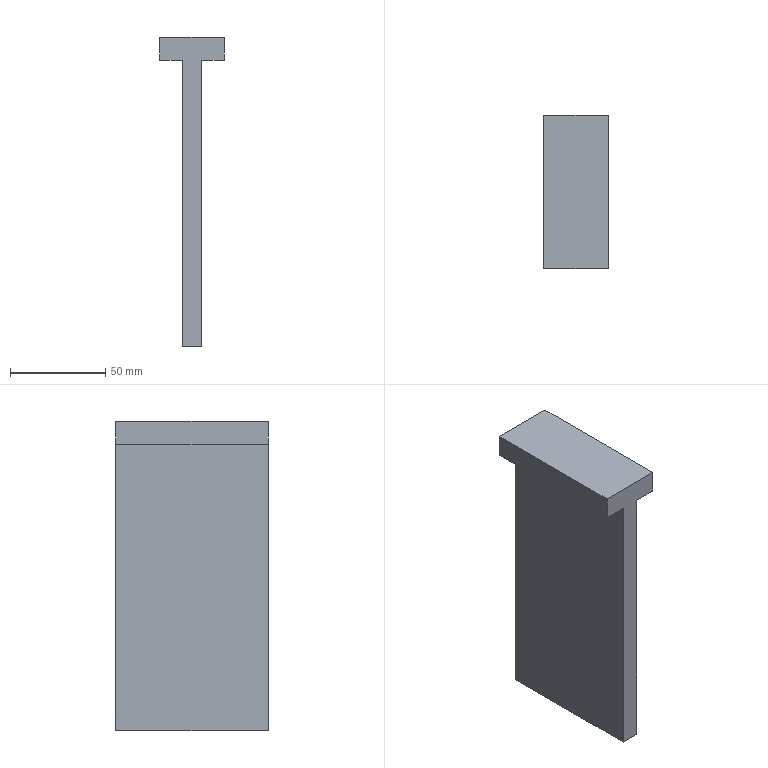Part | SolidWorks | features Extrusion 1, ICE 1, MirrorPattern 1 | 1 solid | 10 faces | box 34 x 80 x 162 mm | volume 152640 mm3 | plane 10
STEP:
#1=CARTESIAN_POINT('',(-5.,-40.,-75.));
#2=VERTEX_POINT('',#1);
#3=CARTESIAN_POINT('',(-5.,40.,-75.));
#4=VERTEX_POINT('',#3);
#5=CARTESIAN_POINT('',(-5.,-40.,-75.));
#6=DIRECTION('',(0.,1.,0.));
#7=VECTOR('',#6,1000.);
#8=LINE('',#5,#7);
#9=EDGE_CURVE('',#2,#4,#8,.T.);
#10=ORIENTED_EDGE('',*,*,#9,.T.);
#11=CARTESIAN_POINT('',(5.,40.,-75.));
#12=VERTEX_POINT('',#11);
#13=CARTESIAN_POINT('',(5.,40.,-75.));
#14=DIRECTION('',(-1.,0.,0.));
#15=VECTOR('',#14,1000.);
#16=LINE('',#13,#15);
#17=EDGE_CURVE('',#12,#4,#16,.T.);
#18=ORIENTED_EDGE('',*,*,#17,.F.);
#19=CARTESIAN_POINT('',(5.,-40.,-75.));
#20=VERTEX_POINT('',#19);
#21=CARTESIAN_POINT('',(5.,-40.,-75.));
#22=DIRECTION('',(0.,1.,0.));
#23=VECTOR('',#22,1000.);
#24=LINE('',#21,#23);
#25=EDGE_CURVE('',#20,#12,#24,.T.);
#26=ORIENTED_EDGE('',*,*,#25,.F.);
#27=CARTESIAN_POINT('',(5.,-40.,-75.));
#28=DIRECTION('',(-1.,0.,0.));
#29=VECTOR('',#28,1000.);
#30=LINE('',#27,#29);
#31=EDGE_CURVE('',#20,#2,#30,.T.);
#32=ORIENTED_EDGE('',*,*,#31,.T.);
#33=EDGE_LOOP('',(#10,#18,#26,#32));
#34=FACE_OUTER_BOUND('',#33,.T.);
#35=CARTESIAN_POINT('',(5.,-40.,-75.));
#36=DIRECTION('',(0.,0.,1.));
#37=DIRECTION('',(1.,0.,0.));
#38=AXIS2_PLACEMENT_3D('',#35,#36,#37);
#39=PLANE('',#38);
#40=ADVANCED_FACE('',(#34),#39,.F.);
#41=CARTESIAN_POINT('',(-5.,40.,75.));
#42=VERTEX_POINT('',#41);
#43=CARTESIAN_POINT('',(-5.,40.,75.));
#44=DIRECTION('',(0.,0.,1.));
#45=VECTOR('',#44,1000.);
#46=LINE('',#43,#45);
#47=EDGE_CURVE('',#4,#42,#46,.T.);
#48=ORIENTED_EDGE('',*,*,#47,.T.);
#49=CARTESIAN_POINT('',(-17.,40.,75.));
#50=VERTEX_POINT('',#49);
#51=CARTESIAN_POINT('',(5.,40.,75.));
#52=DIRECTION('',(1.,0.,0.));
#53=VECTOR('',#52,1000.);
#54=LINE('',#51,#53);
#55=EDGE_CURVE('',#50,#42,#54,.T.);
#56=ORIENTED_EDGE('',*,*,#55,.F.);
#57=CARTESIAN_POINT('',(-17.,40.,87.));
#58=VERTEX_POINT('',#57);
#59=CARTESIAN_POINT('',(-17.,40.,87.));
#60=DIRECTION('',(0.,0.,-1.));
#61=VECTOR('',#60,1000.);
#62=LINE('',#59,#61);
#63=EDGE_CURVE('',#58,#50,#62,.T.);
#64=ORIENTED_EDGE('',*,*,#63,.F.);
#65=CARTESIAN_POINT('',(17.,40.,87.));
#66=VERTEX_POINT('',#65);
#67=CARTESIAN_POINT('',(-5.,40.,87.));
#68=DIRECTION('',(-1.,0.,0.));
#69=VECTOR('',#68,1000.);
#70=LINE('',#67,#69);
#71=EDGE_CURVE('',#66,#58,#70,.T.);
#72=ORIENTED_EDGE('',*,*,#71,.F.);
#73=CARTESIAN_POINT('',(17.,40.,75.));
#74=VERTEX_POINT('',#73);
#75=CARTESIAN_POINT('',(17.,40.,87.));
#76=DIRECTION('',(0.,0.,-1.));
#77=VECTOR('',#76,1000.);
#78=LINE('',#75,#77);
#79=EDGE_CURVE('',#66,#74,#78,.T.);
#80=ORIENTED_EDGE('',*,*,#79,.T.);
#81=CARTESIAN_POINT('',(5.,40.,75.));
#82=VERTEX_POINT('',#81);
#83=CARTESIAN_POINT('',(-5.,40.,75.));
#84=DIRECTION('',(-1.,0.,0.));
#85=VECTOR('',#84,1000.);
#86=LINE('',#83,#85);
#87=EDGE_CURVE('',#74,#82,#86,.T.);
#88=ORIENTED_EDGE('',*,*,#87,.T.);
#89=CARTESIAN_POINT('',(5.,40.,75.));
#90=DIRECTION('',(0.,0.,1.));
#91=VECTOR('',#90,1000.);
#92=LINE('',#89,#91);
#93=EDGE_CURVE('',#12,#82,#92,.T.);
#94=ORIENTED_EDGE('',*,*,#93,.F.);
#95=ORIENTED_EDGE('',*,*,#17,.T.);
#96=EDGE_LOOP('',(#48,#56,#64,#72,#80,#88,#94,#95));
#97=FACE_OUTER_BOUND('',#96,.T.);
#98=CARTESIAN_POINT('',(5.,40.,75.));
#99=DIRECTION('',(0.,-1.,0.));
#100=DIRECTION('',(0.,0.,-1.));
#101=AXIS2_PLACEMENT_3D('',#98,#99,#100);
#102=PLANE('',#101);
#103=ADVANCED_FACE('',(#97),#102,.F.);
#104=CARTESIAN_POINT('',(5.,-40.,75.));
#105=VERTEX_POINT('',#104);
#106=CARTESIAN_POINT('',(5.,-40.,75.));
#107=DIRECTION('',(0.,0.,-1.));
#108=VECTOR('',#107,1000.);
#109=LINE('',#106,#108);
#110=EDGE_CURVE('',#105,#20,#109,.T.);
#111=ORIENTED_EDGE('',*,*,#110,.F.);
#112=CARTESIAN_POINT('',(17.,-40.,75.));
#113=VERTEX_POINT('',#112);
#114=CARTESIAN_POINT('',(-5.,-40.,75.));
#115=DIRECTION('',(1.,0.,0.));
#116=VECTOR('',#115,1000.);
#117=LINE('',#114,#116);
#118=EDGE_CURVE('',#105,#113,#117,.T.);
#119=ORIENTED_EDGE('',*,*,#118,.T.);
#120=CARTESIAN_POINT('',(17.,-40.,87.));
#121=VERTEX_POINT('',#120);
#122=CARTESIAN_POINT('',(17.,-40.,87.));
#123=DIRECTION('',(0.,0.,-1.));
#124=VECTOR('',#123,1000.);
#125=LINE('',#122,#124);
#126=EDGE_CURVE('',#121,#113,#125,.T.);
#127=ORIENTED_EDGE('',*,*,#126,.F.);
#128=CARTESIAN_POINT('',(-17.,-40.,87.));
#129=VERTEX_POINT('',#128);
#130=CARTESIAN_POINT('',(-5.,-40.,87.));
#131=DIRECTION('',(1.,0.,0.));
#132=VECTOR('',#131,1000.);
#133=LINE('',#130,#132);
#134=EDGE_CURVE('',#129,#121,#133,.T.);
#135=ORIENTED_EDGE('',*,*,#134,.F.);
#136=CARTESIAN_POINT('',(-17.,-40.,75.));
#137=VERTEX_POINT('',#136);
#138=CARTESIAN_POINT('',(-17.,-40.,87.));
#139=DIRECTION('',(0.,0.,-1.));
#140=VECTOR('',#139,1000.);
#141=LINE('',#138,#140);
#142=EDGE_CURVE('',#129,#137,#141,.T.);
#143=ORIENTED_EDGE('',*,*,#142,.T.);
#144=CARTESIAN_POINT('',(-5.,-40.,75.));
#145=VERTEX_POINT('',#144);
#146=CARTESIAN_POINT('',(5.,-40.,75.));
#147=DIRECTION('',(-1.,0.,0.));
#148=VECTOR('',#147,1000.);
#149=LINE('',#146,#148);
#150=EDGE_CURVE('',#145,#137,#149,.T.);
#151=ORIENTED_EDGE('',*,*,#150,.F.);
#152=CARTESIAN_POINT('',(-5.,-40.,75.));
#153=DIRECTION('',(0.,0.,-1.));
#154=VECTOR('',#153,1000.);
#155=LINE('',#152,#154);
#156=EDGE_CURVE('',#145,#2,#155,.T.);
#157=ORIENTED_EDGE('',*,*,#156,.T.);
#158=ORIENTED_EDGE('',*,*,#31,.F.);
#159=EDGE_LOOP('',(#111,#119,#127,#135,#143,#151,#157,#158));
#160=FACE_OUTER_BOUND('',#159,.T.);
#161=CARTESIAN_POINT('',(5.,-40.,75.));
#162=DIRECTION('',(0.,1.,0.));
#163=DIRECTION('',(0.,0.,1.));
#164=AXIS2_PLACEMENT_3D('',#161,#162,#163);
#165=PLANE('',#164);
#166=ADVANCED_FACE('',(#160),#165,.F.);
#167=ORIENTED_EDGE('',*,*,#25,.T.);
#168=ORIENTED_EDGE('',*,*,#93,.T.);
#169=CARTESIAN_POINT('',(5.,-40.,75.));
#170=DIRECTION('',(0.,-1.,0.));
#171=VECTOR('',#170,1000.);
#172=LINE('',#169,#171);
#173=EDGE_CURVE('',#82,#105,#172,.T.);
#174=ORIENTED_EDGE('',*,*,#173,.T.);
#175=ORIENTED_EDGE('',*,*,#110,.T.);
#176=EDGE_LOOP('',(#167,#168,#174,#175));
#177=FACE_OUTER_BOUND('',#176,.T.);
#178=CARTESIAN_POINT('',(5.,0.,0.));
#179=DIRECTION('',(-1.,0.,0.));
#180=DIRECTION('',(0.,0.,1.));
#181=AXIS2_PLACEMENT_3D('',#178,#179,#180);
#182=PLANE('',#181);
#183=ADVANCED_FACE('',(#177),#182,.F.);
#184=CARTESIAN_POINT('',(-5.,0.,75.));
#185=DIRECTION('',(0.,-1.,0.));
#186=VECTOR('',#185,1000.);
#187=LINE('',#184,#186);
#188=EDGE_CURVE('',#42,#145,#187,.T.);
#189=ORIENTED_EDGE('',*,*,#188,.F.);
#190=ORIENTED_EDGE('',*,*,#47,.F.);
#191=ORIENTED_EDGE('',*,*,#9,.F.);
#192=ORIENTED_EDGE('',*,*,#156,.F.);
#193=EDGE_LOOP('',(#189,#190,#191,#192));
#194=FACE_OUTER_BOUND('',#193,.T.);
#195=CARTESIAN_POINT('',(-5.,0.,0.));
#196=DIRECTION('',(-1.,0.,0.));
#197=DIRECTION('',(0.,0.,1.));
#198=AXIS2_PLACEMENT_3D('',#195,#196,#197);
#199=PLANE('',#198);
#200=ADVANCED_FACE('',(#194),#199,.T.);
#201=ORIENTED_EDGE('',*,*,#173,.F.);
#202=ORIENTED_EDGE('',*,*,#87,.F.);
#203=CARTESIAN_POINT('',(17.,-40.,75.));
#204=DIRECTION('',(0.,1.,0.));
#205=VECTOR('',#204,1000.);
#206=LINE('',#203,#205);
#207=EDGE_CURVE('',#113,#74,#206,.T.);
#208=ORIENTED_EDGE('',*,*,#207,.F.);
#209=ORIENTED_EDGE('',*,*,#118,.F.);
#210=EDGE_LOOP('',(#201,#202,#208,#209));
#211=FACE_OUTER_BOUND('',#210,.T.);
#212=CARTESIAN_POINT('',(0.,0.,75.));
#213=DIRECTION('',(0.,0.,-1.));
#214=DIRECTION('',(-1.,0.,0.));
#215=AXIS2_PLACEMENT_3D('',#212,#213,#214);
#216=PLANE('',#215);
#217=ADVANCED_FACE('',(#211),#216,.T.);
#218=ORIENTED_EDGE('',*,*,#207,.T.);
#219=ORIENTED_EDGE('',*,*,#79,.F.);
#220=CARTESIAN_POINT('',(17.,-40.,87.));
#221=DIRECTION('',(0.,1.,0.));
#222=VECTOR('',#221,1000.);
#223=LINE('',#220,#222);
#224=EDGE_CURVE('',#121,#66,#223,.T.);
#225=ORIENTED_EDGE('',*,*,#224,.F.);
#226=ORIENTED_EDGE('',*,*,#126,.T.);
#227=EDGE_LOOP('',(#218,#219,#225,#226));
#228=FACE_OUTER_BOUND('',#227,.T.);
#229=CARTESIAN_POINT('',(17.,-40.,87.));
#230=DIRECTION('',(-1.,0.,0.));
#231=DIRECTION('',(0.,0.,1.));
#232=AXIS2_PLACEMENT_3D('',#229,#230,#231);
#233=PLANE('',#232);
#234=ADVANCED_FACE('',(#228),#233,.F.);
#235=ORIENTED_EDGE('',*,*,#71,.T.);
#236=CARTESIAN_POINT('',(-17.,-40.,87.));
#237=DIRECTION('',(0.,1.,0.));
#238=VECTOR('',#237,1000.);
#239=LINE('',#236,#238);
#240=EDGE_CURVE('',#129,#58,#239,.T.);
#241=ORIENTED_EDGE('',*,*,#240,.F.);
#242=ORIENTED_EDGE('',*,*,#134,.T.);
#243=ORIENTED_EDGE('',*,*,#224,.T.);
#244=EDGE_LOOP('',(#235,#241,#242,#243));
#245=FACE_OUTER_BOUND('',#244,.T.);
#246=CARTESIAN_POINT('',(0.,0.,87.));
#247=DIRECTION('',(0.,0.,-1.));
#248=DIRECTION('',(-1.,0.,0.));
#249=AXIS2_PLACEMENT_3D('',#246,#247,#248);
#250=PLANE('',#249);
#251=ADVANCED_FACE('',(#245),#250,.F.);
#252=CARTESIAN_POINT('',(-17.,-40.,75.));
#253=DIRECTION('',(0.,1.,0.));
#254=VECTOR('',#253,1000.);
#255=LINE('',#252,#254);
#256=EDGE_CURVE('',#137,#50,#255,.T.);
#257=ORIENTED_EDGE('',*,*,#256,.F.);
#258=ORIENTED_EDGE('',*,*,#142,.F.);
#259=ORIENTED_EDGE('',*,*,#240,.T.);
#260=ORIENTED_EDGE('',*,*,#63,.T.);
#261=EDGE_LOOP('',(#257,#258,#259,#260));
#262=FACE_OUTER_BOUND('',#261,.T.);
#263=CARTESIAN_POINT('',(-17.,-40.,87.));
#264=DIRECTION('',(-1.,0.,0.));
#265=DIRECTION('',(0.,0.,1.));
#266=AXIS2_PLACEMENT_3D('',#263,#264,#265);
#267=PLANE('',#266);
#268=ADVANCED_FACE('',(#262),#267,.T.);
#269=ORIENTED_EDGE('',*,*,#55,.T.);
#270=ORIENTED_EDGE('',*,*,#188,.T.);
#271=ORIENTED_EDGE('',*,*,#150,.T.);
#272=ORIENTED_EDGE('',*,*,#256,.T.);
#273=EDGE_LOOP('',(#269,#270,#271,#272));
#274=FACE_OUTER_BOUND('',#273,.T.);
#275=CARTESIAN_POINT('',(0.,0.,75.));
#276=DIRECTION('',(0.,0.,-1.));
#277=DIRECTION('',(1.,0.,0.));
#278=AXIS2_PLACEMENT_3D('',#275,#276,#277);
#279=PLANE('',#278);
#280=ADVANCED_FACE('',(#274),#279,.T.);
#281=CLOSED_SHELL('',(#40,#103,#166,#183,#200,#217,#234,#251,#268,#280));
#282=MANIFOLD_SOLID_BREP('',#281);
#283=CARTESIAN_POINT('',(0.,0.,0.));
#284=DIRECTION('',(0.,0.,1.));
#285=DIRECTION('',(1.,0.,0.));
#286=AXIS2_PLACEMENT_3D('',#283,#284,#285);
#287=(LENGTH_UNIT()NAMED_UNIT(*)SI_UNIT(.MILLI.,.METRE.));
#288=UNCERTAINTY_MEASURE_WITH_UNIT(LENGTH_MEASURE(0.00001),#287,'','');
#289=(NAMED_UNIT(*)PLANE_ANGLE_UNIT()SI_UNIT($,.RADIAN.));
#290=(NAMED_UNIT(*)SI_UNIT($,.STERADIAN.)SOLID_ANGLE_UNIT());
#291=(GEOMETRIC_REPRESENTATION_CONTEXT(3)GLOBAL_UNCERTAINTY_ASSIGNED_CONTEXT((#288))GLOBAL_UNIT_ASSIGNED_CONTEXT((#287,#289,#290))REPRESENTATION_CONTEXT('',''));
#292=ADVANCED_BREP_SHAPE_REPRESENTATION('',(#282,#286),#291);